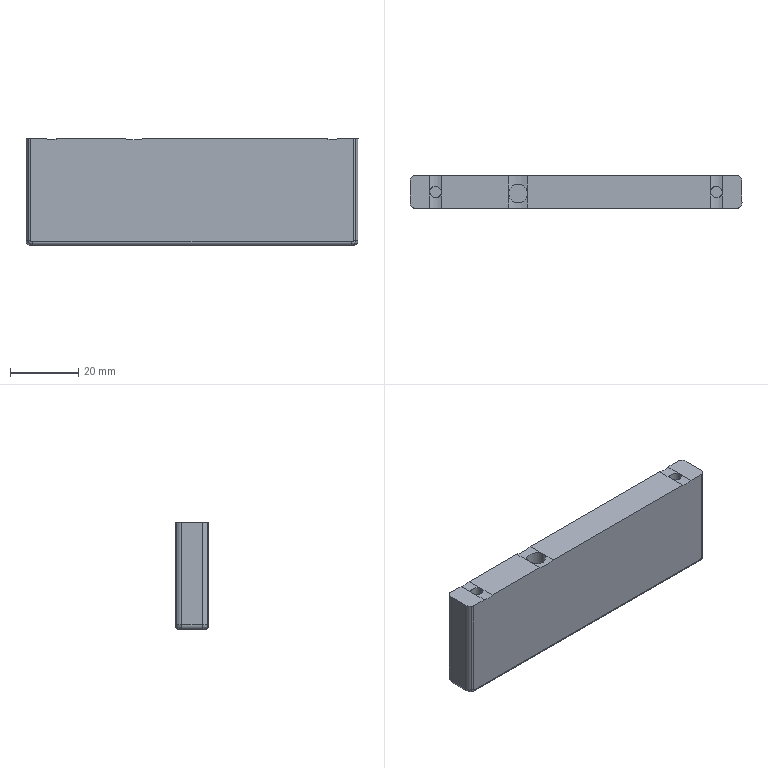Part | SolidWorks | features BaseBody 1 | 1 solid | 46 faces | box 97.4 x 9.6 x 31.25 mm | volume 28550 mm3 | cylinder 26 | plane 12 | spline 8 | commonest cylinder face diameters 2 x6 2.5 x4 3.4 x4 4 x4 10 x4 5.5 x2